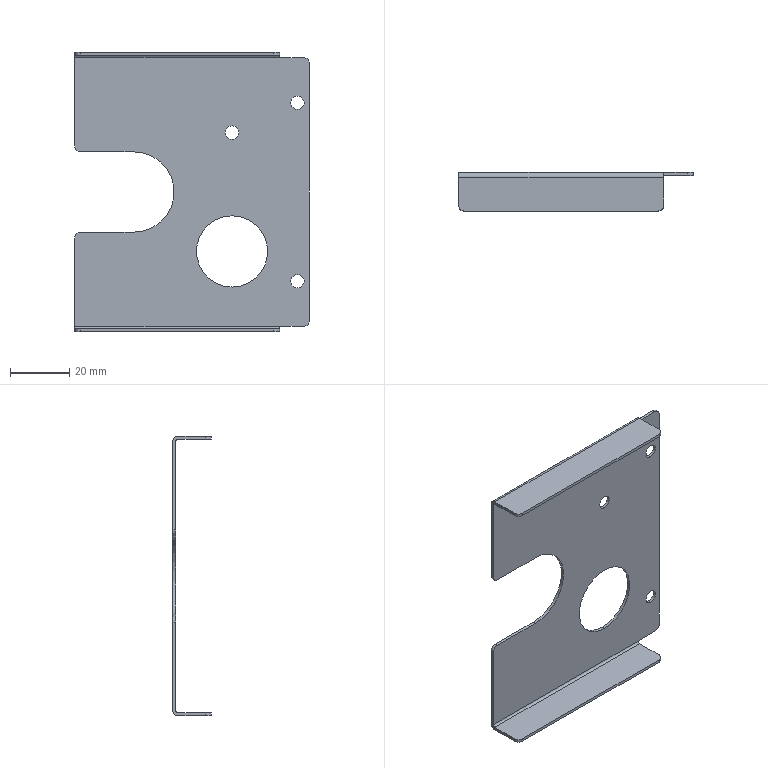Part | SolidWorks | features BaseBody 1 | 1 solid | 38 faces | box 79 x 13 x 94 mm | volume 7641 mm3 | cylinder 21 | plane 17 | commonest cylinder face diameters 4 x8 4.5 x6 1.473 x2 3.473 x2 24 x2 27 x1
STEP:
#1=CARTESIAN_POINT('',(13.5,-1.,-8.));
#2=VERTEX_POINT('',#1);
#3=CARTESIAN_POINT('',(13.5,-1.,-32.));
#4=VERTEX_POINT('',#3);
#5=CARTESIAN_POINT('',(13.5,-1.,-20.));
#6=DIRECTION('',(0.,-1.,0.));
#7=DIRECTION('',(0.,0.,1.));
#8=AXIS2_PLACEMENT_3D('',#5,#6,#7);
#9=CIRCLE('',#8,12.);
#10=EDGE_CURVE('',#2,#4,#9,.T.);
#11=ORIENTED_EDGE('',*,*,#10,.T.);
#12=CARTESIAN_POINT('',(13.5,0.,-32.));
#13=VERTEX_POINT('',#12);
#14=CARTESIAN_POINT('',(13.5,-50.,-32.));
#15=DIRECTION('',(0.,1.,0.));
#16=VECTOR('',#15,1000.);
#17=LINE('',#14,#16);
#18=EDGE_CURVE('',#4,#13,#17,.T.);
#19=ORIENTED_EDGE('',*,*,#18,.T.);
#20=CARTESIAN_POINT('',(13.5,0.,-8.));
#21=VERTEX_POINT('',#20);
#22=CARTESIAN_POINT('',(13.5,0.,-20.));
#23=DIRECTION('',(0.,-1.,0.));
#24=DIRECTION('',(0.,0.,1.));
#25=AXIS2_PLACEMENT_3D('',#22,#23,#24);
#26=CIRCLE('',#25,12.);
#27=EDGE_CURVE('',#21,#13,#26,.T.);
#28=ORIENTED_EDGE('',*,*,#27,.F.);
#29=CARTESIAN_POINT('',(13.5,-50.,-8.));
#30=DIRECTION('',(0.,1.,0.));
#31=VECTOR('',#30,1000.);
#32=LINE('',#29,#31);
#33=EDGE_CURVE('',#2,#21,#32,.T.);
#34=ORIENTED_EDGE('',*,*,#33,.F.);
#35=EDGE_LOOP('',(#11,#19,#28,#34));
#36=FACE_OUTER_BOUND('',#35,.T.);
#37=CARTESIAN_POINT('',(13.5,-50.,-20.));
#38=DIRECTION('',(0.,1.,0.));
#39=DIRECTION('',(0.,0.,1.));
#40=AXIS2_PLACEMENT_3D('',#37,#38,#39);
#41=CYLINDRICAL_SURFACE('',#40,12.);
#42=ADVANCED_FACE('',(#36),#41,.F.);
#43=CARTESIAN_POINT('',(35.5,-1.,-27.75));
#44=VERTEX_POINT('',#43);
#45=CARTESIAN_POINT('',(35.5,-1.,-32.25));
#46=VERTEX_POINT('',#45);
#47=CARTESIAN_POINT('',(35.5,-1.,-30.));
#48=DIRECTION('',(0.,-1.,0.));
#49=DIRECTION('',(0.,0.,1.));
#50=AXIS2_PLACEMENT_3D('',#47,#48,#49);
#51=CIRCLE('',#50,2.25);
#52=EDGE_CURVE('',#44,#46,#51,.T.);
#53=ORIENTED_EDGE('',*,*,#52,.T.);
#54=CARTESIAN_POINT('',(35.5,0.,-32.25));
#55=VERTEX_POINT('',#54);
#56=CARTESIAN_POINT('',(35.5,-50.,-32.25));
#57=DIRECTION('',(0.,1.,0.));
#58=VECTOR('',#57,1000.);
#59=LINE('',#56,#58);
#60=EDGE_CURVE('',#46,#55,#59,.T.);
#61=ORIENTED_EDGE('',*,*,#60,.T.);
#62=CARTESIAN_POINT('',(35.5,0.,-27.75));
#63=VERTEX_POINT('',#62);
#64=CARTESIAN_POINT('',(35.5,0.,-30.));
#65=DIRECTION('',(0.,-1.,0.));
#66=DIRECTION('',(0.,0.,1.));
#67=AXIS2_PLACEMENT_3D('',#64,#65,#66);
#68=CIRCLE('',#67,2.25);
#69=EDGE_CURVE('',#63,#55,#68,.T.);
#70=ORIENTED_EDGE('',*,*,#69,.F.);
#71=CARTESIAN_POINT('',(35.5,-50.,-27.75));
#72=DIRECTION('',(0.,1.,0.));
#73=VECTOR('',#72,1000.);
#74=LINE('',#71,#73);
#75=EDGE_CURVE('',#44,#63,#74,.T.);
#76=ORIENTED_EDGE('',*,*,#75,.F.);
#77=EDGE_LOOP('',(#53,#61,#70,#76));
#78=FACE_OUTER_BOUND('',#77,.T.);
#79=CARTESIAN_POINT('',(35.5,-50.,-30.));
#80=DIRECTION('',(0.,1.,0.));
#81=DIRECTION('',(0.,0.,1.));
#82=AXIS2_PLACEMENT_3D('',#79,#80,#81);
#83=CYLINDRICAL_SURFACE('',#82,2.25);
#84=ADVANCED_FACE('',(#78),#83,.F.);
#85=CARTESIAN_POINT('',(35.5,-1.,32.25));
#86=VERTEX_POINT('',#85);
#87=CARTESIAN_POINT('',(35.5,-1.,27.75));
#88=VERTEX_POINT('',#87);
#89=CARTESIAN_POINT('',(35.5,-1.,30.));
#90=DIRECTION('',(0.,-1.,0.));
#91=DIRECTION('',(0.,0.,1.));
#92=AXIS2_PLACEMENT_3D('',#89,#90,#91);
#93=CIRCLE('',#92,2.25);
#94=EDGE_CURVE('',#86,#88,#93,.T.);
#95=ORIENTED_EDGE('',*,*,#94,.T.);
#96=CARTESIAN_POINT('',(35.5,0.,27.75));
#97=VERTEX_POINT('',#96);
#98=CARTESIAN_POINT('',(35.5,-50.,27.75));
#99=DIRECTION('',(0.,1.,0.));
#100=VECTOR('',#99,1000.);
#101=LINE('',#98,#100);
#102=EDGE_CURVE('',#88,#97,#101,.T.);
#103=ORIENTED_EDGE('',*,*,#102,.T.);
#104=CARTESIAN_POINT('',(35.5,0.,32.25));
#105=VERTEX_POINT('',#104);
#106=CARTESIAN_POINT('',(35.5,0.,30.));
#107=DIRECTION('',(0.,-1.,0.));
#108=DIRECTION('',(0.,0.,1.));
#109=AXIS2_PLACEMENT_3D('',#106,#107,#108);
#110=CIRCLE('',#109,2.25);
#111=EDGE_CURVE('',#105,#97,#110,.T.);
#112=ORIENTED_EDGE('',*,*,#111,.F.);
#113=CARTESIAN_POINT('',(35.5,-50.,32.25));
#114=DIRECTION('',(0.,1.,0.));
#115=VECTOR('',#114,1000.);
#116=LINE('',#113,#115);
#117=EDGE_CURVE('',#86,#105,#116,.T.);
#118=ORIENTED_EDGE('',*,*,#117,.F.);
#119=EDGE_LOOP('',(#95,#103,#112,#118));
#120=FACE_OUTER_BOUND('',#119,.T.);
#121=CARTESIAN_POINT('',(35.5,-50.,30.));
#122=DIRECTION('',(0.,1.,0.));
#123=DIRECTION('',(0.,0.,1.));
#124=AXIS2_PLACEMENT_3D('',#121,#122,#123);
#125=CYLINDRICAL_SURFACE('',#124,2.25);
#126=ADVANCED_FACE('',(#120),#125,.F.);
#127=CARTESIAN_POINT('',(13.5,-1.,22.25));
#128=VERTEX_POINT('',#127);
#129=CARTESIAN_POINT('',(13.5,-1.,17.75));
#130=VERTEX_POINT('',#129);
#131=CARTESIAN_POINT('',(13.5,-1.,20.));
#132=DIRECTION('',(0.,-1.,0.));
#133=DIRECTION('',(0.,0.,1.));
#134=AXIS2_PLACEMENT_3D('',#131,#132,#133);
#135=CIRCLE('',#134,2.25);
#136=EDGE_CURVE('',#128,#130,#135,.T.);
#137=ORIENTED_EDGE('',*,*,#136,.T.);
#138=CARTESIAN_POINT('',(13.5,0.,17.75));
#139=VERTEX_POINT('',#138);
#140=CARTESIAN_POINT('',(13.5,-50.,17.75));
#141=DIRECTION('',(0.,1.,0.));
#142=VECTOR('',#141,1000.);
#143=LINE('',#140,#142);
#144=EDGE_CURVE('',#130,#139,#143,.T.);
#145=ORIENTED_EDGE('',*,*,#144,.T.);
#146=CARTESIAN_POINT('',(13.5,0.,22.25));
#147=VERTEX_POINT('',#146);
#148=CARTESIAN_POINT('',(13.5,0.,20.));
#149=DIRECTION('',(0.,-1.,0.));
#150=DIRECTION('',(0.,0.,1.));
#151=AXIS2_PLACEMENT_3D('',#148,#149,#150);
#152=CIRCLE('',#151,2.25);
#153=EDGE_CURVE('',#147,#139,#152,.T.);
#154=ORIENTED_EDGE('',*,*,#153,.F.);
#155=CARTESIAN_POINT('',(13.5,-50.,22.25));
#156=DIRECTION('',(0.,1.,0.));
#157=VECTOR('',#156,1000.);
#158=LINE('',#155,#157);
#159=EDGE_CURVE('',#128,#147,#158,.T.);
#160=ORIENTED_EDGE('',*,*,#159,.F.);
#161=EDGE_LOOP('',(#137,#145,#154,#160));
#162=FACE_OUTER_BOUND('',#161,.T.);
#163=CARTESIAN_POINT('',(13.5,-50.,20.));
#164=DIRECTION('',(0.,1.,0.));
#165=DIRECTION('',(0.,0.,1.));
#166=AXIS2_PLACEMENT_3D('',#163,#164,#165);
#167=CYLINDRICAL_SURFACE('',#166,2.25);
#168=ADVANCED_FACE('',(#162),#167,.F.);
#169=CARTESIAN_POINT('',(-39.5,-11.,-47.));
#170=VERTEX_POINT('',#169);
#171=CARTESIAN_POINT('',(-37.5,-13.,-47.));
#172=VERTEX_POINT('',#171);
#173=CARTESIAN_POINT('',(-37.5,-11.,-47.));
#174=DIRECTION('',(0.,0.,1.));
#175=DIRECTION('',(0.,-1.,0.));
#176=AXIS2_PLACEMENT_3D('',#173,#174,#175);
#177=CIRCLE('',#176,2.);
#178=EDGE_CURVE('',#170,#172,#177,.T.);
#179=ORIENTED_EDGE('',*,*,#178,.F.);
#180=CARTESIAN_POINT('',(-39.5,-1.737,-47.));
#181=VERTEX_POINT('',#180);
#182=CARTESIAN_POINT('',(-39.5,-1.,-47.));
#183=DIRECTION('',(0.,1.,0.));
#184=VECTOR('',#183,1000.);
#185=LINE('',#182,#184);
#186=EDGE_CURVE('',#170,#181,#185,.T.);
#187=ORIENTED_EDGE('',*,*,#186,.T.);
#188=CARTESIAN_POINT('',(29.5,-1.737,-47.));
#189=VERTEX_POINT('',#188);
#190=CARTESIAN_POINT('',(39.5,-1.737,-47.));
#191=DIRECTION('',(-1.,0.,0.));
#192=VECTOR('',#191,1000.);
#193=LINE('',#190,#192);
#194=EDGE_CURVE('',#189,#181,#193,.T.);
#195=ORIENTED_EDGE('',*,*,#194,.F.);
#196=CARTESIAN_POINT('',(29.5,-11.,-47.));
#197=VERTEX_POINT('',#196);
#198=CARTESIAN_POINT('',(29.5,-1.,-47.));
#199=DIRECTION('',(0.,1.,0.));
#200=VECTOR('',#199,1000.);
#201=LINE('',#198,#200);
#202=EDGE_CURVE('',#197,#189,#201,.T.);
#203=ORIENTED_EDGE('',*,*,#202,.F.);
#204=CARTESIAN_POINT('',(27.5,-13.,-47.));
#205=VERTEX_POINT('',#204);
#206=CARTESIAN_POINT('',(27.5,-11.,-47.));
#207=DIRECTION('',(0.,0.,1.));
#208=DIRECTION('',(0.,1.,0.));
#209=AXIS2_PLACEMENT_3D('',#206,#207,#208);
#210=CIRCLE('',#209,2.);
#211=EDGE_CURVE('',#205,#197,#210,.T.);
#212=ORIENTED_EDGE('',*,*,#211,.F.);
#213=CARTESIAN_POINT('',(-39.5,-13.,-47.));
#214=DIRECTION('',(-1.,0.,0.));
#215=VECTOR('',#214,1000.);
#216=LINE('',#213,#215);
#217=EDGE_CURVE('',#205,#172,#216,.T.);
#218=ORIENTED_EDGE('',*,*,#217,.T.);
#219=EDGE_LOOP('',(#179,#187,#195,#203,#212,#218));
#220=FACE_OUTER_BOUND('',#219,.T.);
#221=CARTESIAN_POINT('',(39.5,-1.,-47.));
#222=DIRECTION('',(0.,0.,1.));
#223=DIRECTION('',(0.,-1.,0.));
#224=AXIS2_PLACEMENT_3D('',#221,#222,#223);
#225=PLANE('',#224);
#226=ADVANCED_FACE('',(#220),#225,.F.);
#227=CARTESIAN_POINT('',(-37.5,-13.,47.));
#228=VERTEX_POINT('',#227);
#229=CARTESIAN_POINT('',(-39.5,-11.,47.));
#230=VERTEX_POINT('',#229);
#231=CARTESIAN_POINT('',(-37.5,-11.,47.));
#232=DIRECTION('',(0.,0.,-1.));
#233=DIRECTION('',(0.,1.,0.));
#234=AXIS2_PLACEMENT_3D('',#231,#232,#233);
#235=CIRCLE('',#234,2.);
#236=EDGE_CURVE('',#228,#230,#235,.T.);
#237=ORIENTED_EDGE('',*,*,#236,.F.);
#238=CARTESIAN_POINT('',(27.5,-13.,47.));
#239=VERTEX_POINT('',#238);
#240=CARTESIAN_POINT('',(39.5,-13.,47.));
#241=DIRECTION('',(1.,0.,0.));
#242=VECTOR('',#241,1000.);
#243=LINE('',#240,#242);
#244=EDGE_CURVE('',#228,#239,#243,.T.);
#245=ORIENTED_EDGE('',*,*,#244,.T.);
#246=CARTESIAN_POINT('',(29.5,-11.,47.));
#247=VERTEX_POINT('',#246);
#248=CARTESIAN_POINT('',(27.5,-11.,47.));
#249=DIRECTION('',(0.,0.,-1.));
#250=DIRECTION('',(0.,-1.,0.));
#251=AXIS2_PLACEMENT_3D('',#248,#249,#250);
#252=CIRCLE('',#251,2.);
#253=EDGE_CURVE('',#247,#239,#252,.T.);
#254=ORIENTED_EDGE('',*,*,#253,.F.);
#255=CARTESIAN_POINT('',(29.5,-1.737,47.));
#256=VERTEX_POINT('',#255);
#257=CARTESIAN_POINT('',(29.5,-13.,47.));
#258=DIRECTION('',(0.,-1.,0.));
#259=VECTOR('',#258,1000.);
#260=LINE('',#257,#259);
#261=EDGE_CURVE('',#256,#247,#260,.T.);
#262=ORIENTED_EDGE('',*,*,#261,.F.);
#263=CARTESIAN_POINT('',(-39.5,-1.737,47.));
#264=VERTEX_POINT('',#263);
#265=CARTESIAN_POINT('',(-39.5,-1.737,47.));
#266=DIRECTION('',(1.,0.,0.));
#267=VECTOR('',#266,1000.);
#268=LINE('',#265,#267);
#269=EDGE_CURVE('',#264,#256,#268,.T.);
#270=ORIENTED_EDGE('',*,*,#269,.F.);
#271=CARTESIAN_POINT('',(-39.5,-13.,47.));
#272=DIRECTION('',(0.,-1.,0.));
#273=VECTOR('',#272,1000.);
#274=LINE('',#271,#273);
#275=EDGE_CURVE('',#264,#230,#274,.T.);
#276=ORIENTED_EDGE('',*,*,#275,.T.);
#277=EDGE_LOOP('',(#237,#245,#254,#262,#270,#276));
#278=FACE_OUTER_BOUND('',#277,.T.);
#279=CARTESIAN_POINT('',(39.5,-13.,47.));
#280=DIRECTION('',(0.,0.,-1.));
#281=DIRECTION('',(0.,-1.,0.));
#282=AXIS2_PLACEMENT_3D('',#279,#280,#281);
#283=PLANE('',#282);
#284=ADVANCED_FACE('',(#278),#283,.F.);
#285=CARTESIAN_POINT('',(-39.5,-11.,-46.));
#286=VERTEX_POINT('',#285);
#287=CARTESIAN_POINT('',(-37.5,-13.,-46.));
#288=VERTEX_POINT('',#287);
#289=CARTESIAN_POINT('',(-37.5,-11.,-46.));
#290=DIRECTION('',(0.,0.,1.));
#291=DIRECTION('',(0.,-1.,0.));
#292=AXIS2_PLACEMENT_3D('',#289,#290,#291);
#293=CIRCLE('',#292,2.);
#294=EDGE_CURVE('',#286,#288,#293,.T.);
#295=ORIENTED_EDGE('',*,*,#294,.F.);
#296=CARTESIAN_POINT('',(-39.5,-11.,-47.));
#297=DIRECTION('',(0.,0.,-1.));
#298=VECTOR('',#297,1000.);
#299=LINE('',#296,#298);
#300=EDGE_CURVE('',#286,#170,#299,.T.);
#301=ORIENTED_EDGE('',*,*,#300,.T.);
#302=ORIENTED_EDGE('',*,*,#178,.T.);
#303=CARTESIAN_POINT('',(-37.5,-13.,-47.));
#304=DIRECTION('',(0.,0.,1.));
#305=VECTOR('',#304,1000.);
#306=LINE('',#303,#305);
#307=EDGE_CURVE('',#172,#288,#306,.T.);
#308=ORIENTED_EDGE('',*,*,#307,.T.);
#309=EDGE_LOOP('',(#295,#301,#302,#308));
#310=FACE_OUTER_BOUND('',#309,.T.);
#311=CARTESIAN_POINT('',(-37.5,-11.,-47.));
#312=DIRECTION('',(0.,0.,1.));
#313=DIRECTION('',(0.,-1.,0.));
#314=AXIS2_PLACEMENT_3D('',#311,#312,#313);
#315=CYLINDRICAL_SURFACE('',#314,2.);
#316=ADVANCED_FACE('',(#310),#315,.T.);
#317=ORIENTED_EDGE('',*,*,#307,.F.);
#318=ORIENTED_EDGE('',*,*,#217,.F.);
#319=CARTESIAN_POINT('',(27.5,-13.,-46.));
#320=VERTEX_POINT('',#319);
#321=CARTESIAN_POINT('',(27.5,-13.,-47.));
#322=DIRECTION('',(0.,0.,-1.));
#323=VECTOR('',#322,1000.);
#324=LINE('',#321,#323);
#325=EDGE_CURVE('',#320,#205,#324,.T.);
#326=ORIENTED_EDGE('',*,*,#325,.F.);
#327=CARTESIAN_POINT('',(39.5,-13.,-46.));
#328=DIRECTION('',(1.,0.,0.));
#329=VECTOR('',#328,1000.);
#330=LINE('',#327,#329);
#331=EDGE_CURVE('',#288,#320,#330,.T.);
#332=ORIENTED_EDGE('',*,*,#331,.F.);
#333=EDGE_LOOP('',(#317,#318,#326,#332));
#334=FACE_OUTER_BOUND('',#333,.T.);
#335=CARTESIAN_POINT('',(-39.5,-13.,-47.));
#336=DIRECTION('',(0.,1.,0.));
#337=DIRECTION('',(0.,0.,-1.));
#338=AXIS2_PLACEMENT_3D('',#335,#336,#337);
#339=PLANE('',#338);
#340=ADVANCED_FACE('',(#334),#339,.F.);
#341=CARTESIAN_POINT('',(29.5,-11.,-46.));
#342=VERTEX_POINT('',#341);
#343=CARTESIAN_POINT('',(27.5,-11.,-46.));
#344=DIRECTION('',(0.,0.,1.));
#345=DIRECTION('',(0.,1.,0.));
#346=AXIS2_PLACEMENT_3D('',#343,#344,#345);
#347=CIRCLE('',#346,2.);
#348=EDGE_CURVE('',#320,#342,#347,.T.);
#349=ORIENTED_EDGE('',*,*,#348,.F.);
#350=ORIENTED_EDGE('',*,*,#325,.T.);
#351=ORIENTED_EDGE('',*,*,#211,.T.);
#352=CARTESIAN_POINT('',(29.5,-11.,-47.));
#353=DIRECTION('',(0.,0.,-1.));
#354=VECTOR('',#353,1000.);
#355=LINE('',#352,#354);
#356=EDGE_CURVE('',#342,#197,#355,.T.);
#357=ORIENTED_EDGE('',*,*,#356,.F.);
#358=EDGE_LOOP('',(#349,#350,#351,#357));
#359=FACE_OUTER_BOUND('',#358,.T.);
#360=CARTESIAN_POINT('',(27.5,-11.,-47.));
#361=DIRECTION('',(0.,0.,-1.));
#362=DIRECTION('',(0.,1.,0.));
#363=AXIS2_PLACEMENT_3D('',#360,#361,#362);
#364=CYLINDRICAL_SURFACE('',#363,2.);
#365=ADVANCED_FACE('',(#359),#364,.T.);
#366=ORIENTED_EDGE('',*,*,#202,.T.);
#367=CARTESIAN_POINT('',(29.5,0.,-45.263));
#368=VERTEX_POINT('',#367);
#369=CARTESIAN_POINT('',(29.5,-1.737,-45.263));
#370=DIRECTION('',(-1.,0.,0.));
#371=DIRECTION('',(0.,0.,-1.));
#372=AXIS2_PLACEMENT_3D('',#369,#370,#371);
#373=CIRCLE('',#372,1.737);
#374=EDGE_CURVE('',#368,#189,#373,.T.);
#375=ORIENTED_EDGE('',*,*,#374,.F.);
#376=CARTESIAN_POINT('',(29.5,-1.,-45.263));
#377=VERTEX_POINT('',#376);
#378=CARTESIAN_POINT('',(29.5,-1.737,-45.263));
#379=DIRECTION('',(0.,1.,0.));
#380=VECTOR('',#379,1000.);
#381=LINE('',#378,#380);
#382=EDGE_CURVE('',#377,#368,#381,.T.);
#383=ORIENTED_EDGE('',*,*,#382,.F.);
#384=CARTESIAN_POINT('',(29.5,-1.737,-46.));
#385=VERTEX_POINT('',#384);
#386=CARTESIAN_POINT('',(29.5,-1.737,-45.263));
#387=DIRECTION('',(1.,0.,0.));
#388=DIRECTION('',(0.,0.,-1.));
#389=AXIS2_PLACEMENT_3D('',#386,#387,#388);
#390=CIRCLE('',#389,0.7366);
#391=EDGE_CURVE('',#385,#377,#390,.T.);
#392=ORIENTED_EDGE('',*,*,#391,.F.);
#393=CARTESIAN_POINT('',(29.5,-1.,-46.));
#394=DIRECTION('',(0.,1.,0.));
#395=VECTOR('',#394,1000.);
#396=LINE('',#393,#395);
#397=EDGE_CURVE('',#342,#385,#396,.T.);
#398=ORIENTED_EDGE('',*,*,#397,.F.);
#399=ORIENTED_EDGE('',*,*,#356,.T.);
#400=EDGE_LOOP('',(#366,#375,#383,#392,#398,#399));
#401=FACE_OUTER_BOUND('',#400,.T.);
#402=CARTESIAN_POINT('',(29.5,-1.,-47.));
#403=DIRECTION('',(1.,0.,0.));
#404=DIRECTION('',(0.,1.,0.));
#405=AXIS2_PLACEMENT_3D('',#402,#403,#404);
#406=PLANE('',#405);
#407=ADVANCED_FACE('',(#401),#406,.T.);
#408=CARTESIAN_POINT('',(-37.5,-13.,46.));
#409=VERTEX_POINT('',#408);
#410=CARTESIAN_POINT('',(-37.5,-13.,47.));
#411=DIRECTION('',(0.,0.,1.));
#412=VECTOR('',#411,1000.);
#413=LINE('',#410,#412);
#414=EDGE_CURVE('',#409,#228,#413,.T.);
#415=ORIENTED_EDGE('',*,*,#414,.F.);
#416=CARTESIAN_POINT('',(27.5,-13.,46.));
#417=VERTEX_POINT('',#416);
#418=CARTESIAN_POINT('',(39.5,-13.,46.));
#419=DIRECTION('',(-1.,0.,0.));
#420=VECTOR('',#419,1000.);
#421=LINE('',#418,#420);
#422=EDGE_CURVE('',#417,#409,#421,.T.);
#423=ORIENTED_EDGE('',*,*,#422,.F.);
#424=CARTESIAN_POINT('',(27.5,-13.,47.));
#425=DIRECTION('',(0.,0.,-1.));
#426=VECTOR('',#425,1000.);
#427=LINE('',#424,#426);
#428=EDGE_CURVE('',#239,#417,#427,.T.);
#429=ORIENTED_EDGE('',*,*,#428,.F.);
#430=ORIENTED_EDGE('',*,*,#244,.F.);
#431=EDGE_LOOP('',(#415,#423,#429,#430));
#432=FACE_OUTER_BOUND('',#431,.T.);
#433=CARTESIAN_POINT('',(39.5,-13.,47.));
#434=DIRECTION('',(0.,1.,0.));
#435=DIRECTION('',(0.,0.,-1.));
#436=AXIS2_PLACEMENT_3D('',#433,#434,#435);
#437=PLANE('',#436);
#438=ADVANCED_FACE('',(#432),#437,.F.);
#439=CARTESIAN_POINT('',(-39.5,-11.,46.));
#440=VERTEX_POINT('',#439);
#441=CARTESIAN_POINT('',(-37.5,-11.,46.));
#442=DIRECTION('',(0.,0.,-1.));
#443=DIRECTION('',(0.,1.,0.));
#444=AXIS2_PLACEMENT_3D('',#441,#442,#443);
#445=CIRCLE('',#444,2.);
#446=EDGE_CURVE('',#409,#440,#445,.T.);
#447=ORIENTED_EDGE('',*,*,#446,.F.);
#448=ORIENTED_EDGE('',*,*,#414,.T.);
#449=ORIENTED_EDGE('',*,*,#236,.T.);
#450=CARTESIAN_POINT('',(-39.5,-11.,47.));
#451=DIRECTION('',(0.,0.,-1.));
#452=VECTOR('',#451,1000.);
#453=LINE('',#450,#452);
#454=EDGE_CURVE('',#230,#440,#453,.T.);
#455=ORIENTED_EDGE('',*,*,#454,.T.);
#456=EDGE_LOOP('',(#447,#448,#449,#455));
#457=FACE_OUTER_BOUND('',#456,.T.);
#458=CARTESIAN_POINT('',(-37.5,-11.,47.));
#459=DIRECTION('',(0.,0.,-1.));
#460=DIRECTION('',(0.,1.,0.));
#461=AXIS2_PLACEMENT_3D('',#458,#459,#460);
#462=CYLINDRICAL_SURFACE('',#461,2.);
#463=ADVANCED_FACE('',(#457),#462,.T.);
#464=CARTESIAN_POINT('',(29.5,-1.737,46.));
#465=VERTEX_POINT('',#464);
#466=CARTESIAN_POINT('',(29.5,-11.,46.));
#467=VERTEX_POINT('',#466);
#468=CARTESIAN_POINT('',(29.5,-13.,46.));
#469=DIRECTION('',(0.,-1.,0.));
#470=VECTOR('',#469,1000.);
#471=LINE('',#468,#470);
#472=EDGE_CURVE('',#465,#467,#471,.T.);
#473=ORIENTED_EDGE('',*,*,#472,.F.);
#474=CARTESIAN_POINT('',(29.5,-1.,45.263));
#475=VERTEX_POINT('',#474);
#476=CARTESIAN_POINT('',(29.5,-1.737,45.263));
#477=DIRECTION('',(1.,0.,0.));
#478=DIRECTION('',(0.,0.,1.));
#479=AXIS2_PLACEMENT_3D('',#476,#477,#478);
#480=CIRCLE('',#479,0.7366);
#481=EDGE_CURVE('',#475,#465,#480,.T.);
#482=ORIENTED_EDGE('',*,*,#481,.F.);
#483=CARTESIAN_POINT('',(29.5,0.,45.263));
#484=VERTEX_POINT('',#483);
#485=CARTESIAN_POINT('',(29.5,-1.737,45.263));
#486=DIRECTION('',(0.,-1.,0.));
#487=VECTOR('',#486,1000.);
#488=LINE('',#485,#487);
#489=EDGE_CURVE('',#484,#475,#488,.T.);
#490=ORIENTED_EDGE('',*,*,#489,.F.);
#491=CARTESIAN_POINT('',(29.5,-1.737,45.263));
#492=DIRECTION('',(-1.,0.,0.));
#493=DIRECTION('',(0.,0.,1.));
#494=AXIS2_PLACEMENT_3D('',#491,#492,#493);
#495=CIRCLE('',#494,1.737);
#496=EDGE_CURVE('',#256,#484,#495,.T.);
#497=ORIENTED_EDGE('',*,*,#496,.F.);
#498=ORIENTED_EDGE('',*,*,#261,.T.);
#499=CARTESIAN_POINT('',(29.5,-11.,47.));
#500=DIRECTION('',(0.,0.,1.));
#501=VECTOR('',#500,1000.);
#502=LINE('',#499,#501);
#503=EDGE_CURVE('',#467,#247,#502,.T.);
#504=ORIENTED_EDGE('',*,*,#503,.F.);
#505=EDGE_LOOP('',(#473,#482,#490,#497,#498,#504));
#506=FACE_OUTER_BOUND('',#505,.T.);
#507=CARTESIAN_POINT('',(29.5,-13.,47.));
#508=DIRECTION('',(1.,0.,0.));
#509=DIRECTION('',(0.,1.,0.));
#510=AXIS2_PLACEMENT_3D('',#507,#508,#509);
#511=PLANE('',#510);
#512=ADVANCED_FACE('',(#506),#511,.T.);
#513=CARTESIAN_POINT('',(27.5,-11.,46.));
#514=DIRECTION('',(0.,0.,-1.));
#515=DIRECTION('',(0.,-1.,0.));
#516=AXIS2_PLACEMENT_3D('',#513,#514,#515);
#517=CIRCLE('',#516,2.);
#518=EDGE_CURVE('',#467,#417,#517,.T.);
#519=ORIENTED_EDGE('',*,*,#518,.F.);
#520=ORIENTED_EDGE('',*,*,#503,.T.);
#521=ORIENTED_EDGE('',*,*,#253,.T.);
#522=ORIENTED_EDGE('',*,*,#428,.T.);
#523=EDGE_LOOP('',(#519,#520,#521,#522));
#524=FACE_OUTER_BOUND('',#523,.T.);
#525=CARTESIAN_POINT('',(27.5,-11.,47.));
#526=DIRECTION('',(0.,0.,1.));
#527=DIRECTION('',(0.,-1.,0.));
#528=AXIS2_PLACEMENT_3D('',#525,#526,#527);
#529=CYLINDRICAL_SURFACE('',#528,2.);
#530=ADVANCED_FACE('',(#524),#529,.T.);
#531=ORIENTED_EDGE('',*,*,#194,.T.);
#532=CARTESIAN_POINT('',(-39.5,0.,-45.263));
#533=VERTEX_POINT('',#532);
#534=CARTESIAN_POINT('',(-39.5,-1.737,-45.263));
#535=DIRECTION('',(1.,0.,0.));
#536=DIRECTION('',(0.,0.,-1.));
#537=AXIS2_PLACEMENT_3D('',#534,#535,#536);
#538=CIRCLE('',#537,1.737);
#539=EDGE_CURVE('',#181,#533,#538,.T.);
#540=ORIENTED_EDGE('',*,*,#539,.T.);
#541=CARTESIAN_POINT('',(39.5,0.,-45.263));
#542=DIRECTION('',(-1.,0.,0.));
#543=VECTOR('',#542,1000.);
#544=LINE('',#541,#543);
#545=EDGE_CURVE('',#368,#533,#544,.T.);
#546=ORIENTED_EDGE('',*,*,#545,.F.);
#547=ORIENTED_EDGE('',*,*,#374,.T.);
#548=EDGE_LOOP('',(#531,#540,#546,#547));
#549=FACE_OUTER_BOUND('',#548,.T.);
#550=CARTESIAN_POINT('',(39.5,-1.737,-45.263));
#551=DIRECTION('',(1.,0.,0.));
#552=DIRECTION('',(0.,0.,-1.));
#553=AXIS2_PLACEMENT_3D('',#550,#551,#552);
#554=CYLINDRICAL_SURFACE('',#553,1.737);
#555=ADVANCED_FACE('',(#549),#554,.T.);
#556=CARTESIAN_POINT('',(-39.5,0.,45.263));
#557=VERTEX_POINT('',#556);
#558=CARTESIAN_POINT('',(39.5,0.,45.263));
#559=DIRECTION('',(1.,0.,0.));
#560=VECTOR('',#559,1000.);
#561=LINE('',#558,#560);
#562=EDGE_CURVE('',#557,#484,#561,.T.);
#563=ORIENTED_EDGE('',*,*,#562,.F.);
#564=CARTESIAN_POINT('',(-39.5,-1.737,45.263));
#565=DIRECTION('',(1.,0.,0.));
#566=DIRECTION('',(0.,0.,1.));
#567=AXIS2_PLACEMENT_3D('',#564,#565,#566);
#568=CIRCLE('',#567,1.737);
#569=EDGE_CURVE('',#557,#264,#568,.T.);
#570=ORIENTED_EDGE('',*,*,#569,.T.);
#571=ORIENTED_EDGE('',*,*,#269,.T.);
#572=ORIENTED_EDGE('',*,*,#496,.T.);
#573=EDGE_LOOP('',(#563,#570,#571,#572));
#574=FACE_OUTER_BOUND('',#573,.T.);
#575=CARTESIAN_POINT('',(-39.5,-1.737,45.263));
#576=DIRECTION('',(-1.,0.,0.));
#577=DIRECTION('',(0.,0.,1.));
#578=AXIS2_PLACEMENT_3D('',#575,#576,#577);
#579=CYLINDRICAL_SURFACE('',#578,1.737);
#580=ADVANCED_FACE('',(#574),#579,.T.);
#581=ORIENTED_EDGE('',*,*,#397,.T.);
#582=CARTESIAN_POINT('',(-39.5,-1.737,-46.));
#583=VERTEX_POINT('',#582);
#584=CARTESIAN_POINT('',(39.5,-1.737,-46.));
#585=DIRECTION('',(-1.,0.,0.));
#586=VECTOR('',#585,1000.);
#587=LINE('',#584,#586);
#588=EDGE_CURVE('',#385,#583,#587,.T.);
#589=ORIENTED_EDGE('',*,*,#588,.T.);
#590=CARTESIAN_POINT('',(-39.5,-1.,-46.));
#591=DIRECTION('',(0.,-1.,0.));
#592=VECTOR('',#591,1000.);
#593=LINE('',#590,#592);
#594=EDGE_CURVE('',#583,#286,#593,.T.);
#595=ORIENTED_EDGE('',*,*,#594,.T.);
#596=ORIENTED_EDGE('',*,*,#294,.T.);
#597=ORIENTED_EDGE('',*,*,#331,.T.);
#598=ORIENTED_EDGE('',*,*,#348,.T.);
#599=EDGE_LOOP('',(#581,#589,#595,#596,#597,#598));
#600=FACE_OUTER_BOUND('',#599,.T.);
#601=CARTESIAN_POINT('',(39.5,-1.,-46.));
#602=DIRECTION('',(0.,0.,1.));
#603=DIRECTION('',(0.,-1.,0.));
#604=AXIS2_PLACEMENT_3D('',#601,#602,#603);
#605=PLANE('',#604);
#606=ADVANCED_FACE('',(#600),#605,.T.);
#607=ORIENTED_EDGE('',*,*,#472,.T.);
#608=ORIENTED_EDGE('',*,*,#518,.T.);
#609=ORIENTED_EDGE('',*,*,#422,.T.);
#610=ORIENTED_EDGE('',*,*,#446,.T.);
#611=CARTESIAN_POINT('',(-39.5,-1.737,46.));
#612=VERTEX_POINT('',#611);
#613=CARTESIAN_POINT('',(-39.5,-13.,46.));
#614=DIRECTION('',(0.,1.,0.));
#615=VECTOR('',#614,1000.);
#616=LINE('',#613,#615);
#617=EDGE_CURVE('',#440,#612,#616,.T.);
#618=ORIENTED_EDGE('',*,*,#617,.T.);
#619=CARTESIAN_POINT('',(-39.5,-1.737,46.));
#620=DIRECTION('',(1.,0.,0.));
#621=VECTOR('',#620,1000.);
#622=LINE('',#619,#621);
#623=EDGE_CURVE('',#612,#465,#622,.T.);
#624=ORIENTED_EDGE('',*,*,#623,.T.);
#625=EDGE_LOOP('',(#607,#608,#609,#610,#618,#624));
#626=FACE_OUTER_BOUND('',#625,.T.);
#627=CARTESIAN_POINT('',(39.5,-13.,46.));
#628=DIRECTION('',(0.,0.,-1.));
#629=DIRECTION('',(0.,-1.,0.));
#630=AXIS2_PLACEMENT_3D('',#627,#628,#629);
#631=PLANE('',#630);
#632=ADVANCED_FACE('',(#626),#631,.T.);
#633=ORIENTED_EDGE('',*,*,#153,.T.);
#634=CARTESIAN_POINT('',(13.5,0.,20.));
#635=DIRECTION('',(0.,-1.,0.));
#636=DIRECTION('',(0.,0.,1.));
#637=AXIS2_PLACEMENT_3D('',#634,#635,#636);
#638=CIRCLE('',#637,2.25);
#639=EDGE_CURVE('',#139,#147,#638,.T.);
#640=ORIENTED_EDGE('',*,*,#639,.T.);
#641=EDGE_LOOP('',(#633,#640));
#642=FACE_BOUND('',#641,.T.);
#643=ORIENTED_EDGE('',*,*,#111,.T.);
#644=CARTESIAN_POINT('',(35.5,0.,30.));
#645=DIRECTION('',(0.,-1.,0.));
#646=DIRECTION('',(0.,0.,1.));
#647=AXIS2_PLACEMENT_3D('',#644,#645,#646);
#648=CIRCLE('',#647,2.25);
#649=EDGE_CURVE('',#97,#105,#648,.T.);
#650=ORIENTED_EDGE('',*,*,#649,.T.);
#651=EDGE_LOOP('',(#643,#650));
#652=FACE_BOUND('',#651,.T.);
#653=ORIENTED_EDGE('',*,*,#69,.T.);
#654=CARTESIAN_POINT('',(35.5,0.,-30.));
#655=DIRECTION('',(0.,-1.,0.));
#656=DIRECTION('',(0.,0.,1.));
#657=AXIS2_PLACEMENT_3D('',#654,#655,#656);
#658=CIRCLE('',#657,2.25);
#659=EDGE_CURVE('',#55,#63,#658,.T.);
#660=ORIENTED_EDGE('',*,*,#659,.T.);
#661=EDGE_LOOP('',(#653,#660));
#662=FACE_BOUND('',#661,.T.);
#663=ORIENTED_EDGE('',*,*,#27,.T.);
#664=CARTESIAN_POINT('',(13.5,0.,-20.));
#665=DIRECTION('',(0.,-1.,0.));
#666=DIRECTION('',(0.,0.,1.));
#667=AXIS2_PLACEMENT_3D('',#664,#665,#666);
#668=CIRCLE('',#667,12.);
#669=EDGE_CURVE('',#13,#21,#668,.T.);
#670=ORIENTED_EDGE('',*,*,#669,.T.);
#671=EDGE_LOOP('',(#663,#670));
#672=FACE_BOUND('',#671,.T.);
#673=CARTESIAN_POINT('',(-39.5,0.,15.5));
#674=VERTEX_POINT('',#673);
#675=CARTESIAN_POINT('',(-39.5,0.,-47.));
#676=DIRECTION('',(0.,0.,-1.));
#677=VECTOR('',#676,1000.);
#678=LINE('',#675,#677);
#679=EDGE_CURVE('',#557,#674,#678,.T.);
#680=ORIENTED_EDGE('',*,*,#679,.F.);
#681=ORIENTED_EDGE('',*,*,#562,.T.);
#682=CARTESIAN_POINT('',(37.5,0.,45.263));
#683=VERTEX_POINT('',#682);
#684=CARTESIAN_POINT('',(34.5,0.,45.263));
#685=DIRECTION('',(1.,0.,0.));
#686=VECTOR('',#685,1000.);
#687=LINE('',#684,#686);
#688=EDGE_CURVE('',#484,#683,#687,.T.);
#689=ORIENTED_EDGE('',*,*,#688,.T.);
#690=CARTESIAN_POINT('',(39.5,0.,43.263));
#691=VERTEX_POINT('',#690);
#692=CARTESIAN_POINT('',(37.5,0.,43.263));
#693=DIRECTION('',(0.,-1.,0.));
#694=DIRECTION('',(0.,0.,1.));
#695=AXIS2_PLACEMENT_3D('',#692,#693,#694);
#696=CIRCLE('',#695,2.);
#697=EDGE_CURVE('',#691,#683,#696,.T.);
#698=ORIENTED_EDGE('',*,*,#697,.F.);
#699=CARTESIAN_POINT('',(39.5,0.,-43.263));
#700=VERTEX_POINT('',#699);
#701=CARTESIAN_POINT('',(39.5,0.,-47.));
#702=DIRECTION('',(0.,0.,-1.));
#703=VECTOR('',#702,1000.);
#704=LINE('',#701,#703);
#705=EDGE_CURVE('',#691,#700,#704,.T.);
#706=ORIENTED_EDGE('',*,*,#705,.T.);
#707=CARTESIAN_POINT('',(37.5,0.,-45.263));
#708=VERTEX_POINT('',#707);
#709=CARTESIAN_POINT('',(37.5,0.,-43.263));
#710=DIRECTION('',(0.,-1.,0.));
#711=DIRECTION('',(0.,0.,1.));
#712=AXIS2_PLACEMENT_3D('',#709,#710,#711);
#713=CIRCLE('',#712,2.);
#714=EDGE_CURVE('',#708,#700,#713,.T.);
#715=ORIENTED_EDGE('',*,*,#714,.F.);
#716=CARTESIAN_POINT('',(34.5,0.,-45.263));
#717=DIRECTION('',(-1.,0.,0.));
#718=VECTOR('',#717,1000.);
#719=LINE('',#716,#718);
#720=EDGE_CURVE('',#708,#368,#719,.T.);
#721=ORIENTED_EDGE('',*,*,#720,.T.);
#722=ORIENTED_EDGE('',*,*,#545,.T.);
#723=CARTESIAN_POINT('',(-39.5,0.,-15.5));
#724=VERTEX_POINT('',#723);
#725=CARTESIAN_POINT('',(-39.5,0.,-47.));
#726=DIRECTION('',(0.,0.,-1.));
#727=VECTOR('',#726,1000.);
#728=LINE('',#725,#727);
#729=EDGE_CURVE('',#724,#533,#728,.T.);
#730=ORIENTED_EDGE('',*,*,#729,.F.);
#731=CARTESIAN_POINT('',(-37.5,0.,-13.5));
#732=VERTEX_POINT('',#731);
#733=CARTESIAN_POINT('',(-37.5,0.,-15.5));
#734=DIRECTION('',(0.,-1.,0.));
#735=DIRECTION('',(0.,0.,1.));
#736=AXIS2_PLACEMENT_3D('',#733,#734,#735);
#737=CIRCLE('',#736,2.);
#738=EDGE_CURVE('',#732,#724,#737,.T.);
#739=ORIENTED_EDGE('',*,*,#738,.F.);
#740=CARTESIAN_POINT('',(-19.5,0.,-13.5));
#741=VERTEX_POINT('',#740);
#742=CARTESIAN_POINT('',(-39.5,0.,-13.5));
#743=DIRECTION('',(1.,0.,0.));
#744=VECTOR('',#743,1000.);
#745=LINE('',#742,#744);
#746=EDGE_CURVE('',#732,#741,#745,.T.);
#747=ORIENTED_EDGE('',*,*,#746,.T.);
#748=CARTESIAN_POINT('',(-19.5,0.,13.5));
#749=VERTEX_POINT('',#748);
#750=CARTESIAN_POINT('',(-19.5,0.,0.));
#751=DIRECTION('',(0.,-1.,0.));
#752=DIRECTION('',(0.,0.,1.));
#753=AXIS2_PLACEMENT_3D('',#750,#751,#752);
#754=CIRCLE('',#753,13.5);
#755=EDGE_CURVE('',#741,#749,#754,.T.);
#756=ORIENTED_EDGE('',*,*,#755,.T.);
#757=CARTESIAN_POINT('',(-37.5,0.,13.5));
#758=VERTEX_POINT('',#757);
#759=CARTESIAN_POINT('',(-19.5,0.,13.5));
#760=DIRECTION('',(-1.,0.,0.));
#761=VECTOR('',#760,1000.);
#762=LINE('',#759,#761);
#763=EDGE_CURVE('',#749,#758,#762,.T.);
#764=ORIENTED_EDGE('',*,*,#763,.T.);
#765=CARTESIAN_POINT('',(-37.5,0.,15.5));
#766=DIRECTION('',(0.,-1.,0.));
#767=DIRECTION('',(0.,0.,-1.));
#768=AXIS2_PLACEMENT_3D('',#765,#766,#767);
#769=CIRCLE('',#768,2.);
#770=EDGE_CURVE('',#674,#758,#769,.T.);
#771=ORIENTED_EDGE('',*,*,#770,.F.);
#772=EDGE_LOOP('',(#680,#681,#689,#698,#706,#715,#721,#722,#730,#739,#747,#756,#764,#771));
#773=FACE_OUTER_BOUND('',#772,.T.);
#774=CARTESIAN_POINT('',(39.5,0.,47.));
#775=DIRECTION('',(0.,1.,0.));
#776=DIRECTION('',(1.,0.,0.));
#777=AXIS2_PLACEMENT_3D('',#774,#775,#776);
#778=PLANE('',#777);
#779=ADVANCED_FACE('',(#642,#652,#662,#672,#773),#778,.T.);
#780=ORIENTED_EDGE('',*,*,#714,.T.);
#781=CARTESIAN_POINT('',(39.5,-1.,-43.263));
#782=VERTEX_POINT('',#781);
#783=CARTESIAN_POINT('',(39.5,-1.,-43.263));
#784=DIRECTION('',(0.,-1.,0.));
#785=VECTOR('',#784,1000.);
#786=LINE('',#783,#785);
#787=EDGE_CURVE('',#700,#782,#786,.T.);
#788=ORIENTED_EDGE('',*,*,#787,.T.);
#789=CARTESIAN_POINT('',(37.5,-1.,-45.263));
#790=VERTEX_POINT('',#789);
#791=CARTESIAN_POINT('',(37.5,-1.,-43.263));
#792=DIRECTION('',(0.,1.,0.));
#793=DIRECTION('',(0.,0.,1.));
#794=AXIS2_PLACEMENT_3D('',#791,#792,#793);
#795=CIRCLE('',#794,2.);
#796=EDGE_CURVE('',#782,#790,#795,.T.);
#797=ORIENTED_EDGE('',*,*,#796,.T.);
#798=CARTESIAN_POINT('',(37.5,-1.,-45.263));
#799=DIRECTION('',(0.,1.,0.));
#800=VECTOR('',#799,1000.);
#801=LINE('',#798,#800);
#802=EDGE_CURVE('',#790,#708,#801,.T.);
#803=ORIENTED_EDGE('',*,*,#802,.T.);
#804=EDGE_LOOP('',(#780,#788,#797,#803));
#805=FACE_OUTER_BOUND('',#804,.T.);
#806=CARTESIAN_POINT('',(37.5,-1.,-43.263));
#807=DIRECTION('',(0.,1.,0.));
#808=DIRECTION('',(0.,0.,1.));
#809=AXIS2_PLACEMENT_3D('',#806,#807,#808);
#810=CYLINDRICAL_SURFACE('',#809,2.);
#811=ADVANCED_FACE('',(#805),#810,.T.);
#812=ORIENTED_EDGE('',*,*,#802,.F.);
#813=CARTESIAN_POINT('',(39.5,-1.,-45.263));
#814=DIRECTION('',(-1.,0.,0.));
#815=VECTOR('',#814,1000.);
#816=LINE('',#813,#815);
#817=EDGE_CURVE('',#790,#377,#816,.T.);
#818=ORIENTED_EDGE('',*,*,#817,.T.);
#819=ORIENTED_EDGE('',*,*,#382,.T.);
#820=ORIENTED_EDGE('',*,*,#720,.F.);
#821=EDGE_LOOP('',(#812,#818,#819,#820));
#822=FACE_OUTER_BOUND('',#821,.T.);
#823=CARTESIAN_POINT('',(34.5,-1.,-45.263));
#824=DIRECTION('',(0.,0.,1.));
#825=DIRECTION('',(1.,0.,0.));
#826=AXIS2_PLACEMENT_3D('',#823,#824,#825);
#827=PLANE('',#826);
#828=ADVANCED_FACE('',(#822),#827,.F.);
#829=CARTESIAN_POINT('',(-39.5,-1.,-45.263));
#830=VERTEX_POINT('',#829);
#831=CARTESIAN_POINT('',(39.5,-1.,-45.263));
#832=DIRECTION('',(-1.,0.,0.));
#833=VECTOR('',#832,1000.);
#834=LINE('',#831,#833);
#835=EDGE_CURVE('',#377,#830,#834,.T.);
#836=ORIENTED_EDGE('',*,*,#835,.T.);
#837=CARTESIAN_POINT('',(-39.5,-1.737,-45.263));
#838=DIRECTION('',(1.,0.,0.));
#839=DIRECTION('',(0.,0.,-1.));
#840=AXIS2_PLACEMENT_3D('',#837,#838,#839);
#841=CIRCLE('',#840,0.7366);
#842=EDGE_CURVE('',#583,#830,#841,.T.);
#843=ORIENTED_EDGE('',*,*,#842,.F.);
#844=ORIENTED_EDGE('',*,*,#588,.F.);
#845=ORIENTED_EDGE('',*,*,#391,.T.);
#846=EDGE_LOOP('',(#836,#843,#844,#845));
#847=FACE_OUTER_BOUND('',#846,.T.);
#848=CARTESIAN_POINT('',(39.5,-1.737,-45.263));
#849=DIRECTION('',(1.,0.,0.));
#850=DIRECTION('',(0.,0.,-1.));
#851=AXIS2_PLACEMENT_3D('',#848,#849,#850);
#852=CYLINDRICAL_SURFACE('',#851,0.7366);
#853=ADVANCED_FACE('',(#847),#852,.F.);
#854=ORIENTED_EDGE('',*,*,#729,.T.);
#855=ORIENTED_EDGE('',*,*,#539,.F.);
#856=ORIENTED_EDGE('',*,*,#186,.F.);
#857=ORIENTED_EDGE('',*,*,#300,.F.);
#858=ORIENTED_EDGE('',*,*,#594,.F.);
#859=ORIENTED_EDGE('',*,*,#842,.T.);
#860=CARTESIAN_POINT('',(-39.5,-1.,-15.5));
#861=VERTEX_POINT('',#860);
#862=CARTESIAN_POINT('',(-39.5,-1.,47.));
#863=DIRECTION('',(0.,0.,1.));
#864=VECTOR('',#863,1000.);
#865=LINE('',#862,#864);
#866=EDGE_CURVE('',#830,#861,#865,.T.);
#867=ORIENTED_EDGE('',*,*,#866,.T.);
#868=CARTESIAN_POINT('',(-39.5,-50.,-15.5));
#869=DIRECTION('',(0.,-1.,0.));
#870=VECTOR('',#869,1000.);
#871=LINE('',#868,#870);
#872=EDGE_CURVE('',#724,#861,#871,.T.);
#873=ORIENTED_EDGE('',*,*,#872,.F.);
#874=EDGE_LOOP('',(#854,#855,#856,#857,#858,#859,#867,#873));
#875=FACE_OUTER_BOUND('',#874,.T.);
#876=CARTESIAN_POINT('',(-39.5,-1.,-47.));
#877=DIRECTION('',(-1.,0.,0.));
#878=DIRECTION('',(0.,0.,1.));
#879=AXIS2_PLACEMENT_3D('',#876,#877,#878);
#880=PLANE('',#879);
#881=ADVANCED_FACE('',(#875),#880,.T.);
#882=CARTESIAN_POINT('',(-37.5,-1.,-13.5));
#883=VERTEX_POINT('',#882);
#884=CARTESIAN_POINT('',(-37.5,-1.,-15.5));
#885=DIRECTION('',(0.,1.,0.));
#886=DIRECTION('',(0.,0.,1.));
#887=AXIS2_PLACEMENT_3D('',#884,#885,#886);
#888=CIRCLE('',#887,2.);
#889=EDGE_CURVE('',#861,#883,#888,.T.);
#890=ORIENTED_EDGE('',*,*,#889,.T.);
#891=CARTESIAN_POINT('',(-37.5,-50.,-13.5));
#892=DIRECTION('',(0.,1.,0.));
#893=VECTOR('',#892,1000.);
#894=LINE('',#891,#893);
#895=EDGE_CURVE('',#883,#732,#894,.T.);
#896=ORIENTED_EDGE('',*,*,#895,.T.);
#897=ORIENTED_EDGE('',*,*,#738,.T.);
#898=ORIENTED_EDGE('',*,*,#872,.T.);
#899=EDGE_LOOP('',(#890,#896,#897,#898));
#900=FACE_OUTER_BOUND('',#899,.T.);
#901=CARTESIAN_POINT('',(-37.5,-50.,-15.5));
#902=DIRECTION('',(0.,1.,0.));
#903=DIRECTION('',(0.,0.,1.));
#904=AXIS2_PLACEMENT_3D('',#901,#902,#903);
#905=CYLINDRICAL_SURFACE('',#904,2.);
#906=ADVANCED_FACE('',(#900),#905,.T.);
#907=ORIENTED_EDGE('',*,*,#895,.F.);
#908=CARTESIAN_POINT('',(-19.5,-1.,-13.5));
#909=VERTEX_POINT('',#908);
#910=CARTESIAN_POINT('',(39.5,-1.,-13.5));
#911=DIRECTION('',(1.,0.,0.));
#912=VECTOR('',#911,1000.);
#913=LINE('',#910,#912);
#914=EDGE_CURVE('',#883,#909,#913,.T.);
#915=ORIENTED_EDGE('',*,*,#914,.T.);
#916=CARTESIAN_POINT('',(-19.5,-50.,-13.5));
#917=DIRECTION('',(0.,1.,0.));
#918=VECTOR('',#917,1000.);
#919=LINE('',#916,#918);
#920=EDGE_CURVE('',#909,#741,#919,.T.);
#921=ORIENTED_EDGE('',*,*,#920,.T.);
#922=ORIENTED_EDGE('',*,*,#746,.F.);
#923=EDGE_LOOP('',(#907,#915,#921,#922));
#924=FACE_OUTER_BOUND('',#923,.T.);
#925=CARTESIAN_POINT('',(-39.5,-50.,-13.5));
#926=DIRECTION('',(0.,0.,-1.));
#927=DIRECTION('',(0.,-1.,0.));
#928=AXIS2_PLACEMENT_3D('',#925,#926,#927);
#929=PLANE('',#928);
#930=ADVANCED_FACE('',(#924),#929,.F.);
#931=ORIENTED_EDGE('',*,*,#755,.F.);
#932=ORIENTED_EDGE('',*,*,#920,.F.);
#933=CARTESIAN_POINT('',(-19.5,-1.,13.5));
#934=VERTEX_POINT('',#933);
#935=CARTESIAN_POINT('',(-19.5,-1.,0.));
#936=DIRECTION('',(0.,-1.,0.));
#937=DIRECTION('',(0.,0.,1.));
#938=AXIS2_PLACEMENT_3D('',#935,#936,#937);
#939=CIRCLE('',#938,13.5);
#940=EDGE_CURVE('',#909,#934,#939,.T.);
#941=ORIENTED_EDGE('',*,*,#940,.T.);
#942=CARTESIAN_POINT('',(-19.5,-50.,13.5));
#943=DIRECTION('',(0.,1.,0.));
#944=VECTOR('',#943,1000.);
#945=LINE('',#942,#944);
#946=EDGE_CURVE('',#934,#749,#945,.T.);
#947=ORIENTED_EDGE('',*,*,#946,.T.);
#948=EDGE_LOOP('',(#931,#932,#941,#947));
#949=FACE_OUTER_BOUND('',#948,.T.);
#950=CARTESIAN_POINT('',(-19.5,-50.,0.));
#951=DIRECTION('',(0.,1.,0.));
#952=DIRECTION('',(0.,0.,1.));
#953=AXIS2_PLACEMENT_3D('',#950,#951,#952);
#954=CYLINDRICAL_SURFACE('',#953,13.5);
#955=ADVANCED_FACE('',(#949),#954,.F.);
#956=CARTESIAN_POINT('',(-37.5,-1.,13.5));
#957=VERTEX_POINT('',#956);
#958=CARTESIAN_POINT('',(-37.5,-50.,13.5));
#959=DIRECTION('',(0.,-1.,0.));
#960=VECTOR('',#959,1000.);
#961=LINE('',#958,#960);
#962=EDGE_CURVE('',#758,#957,#961,.T.);
#963=ORIENTED_EDGE('',*,*,#962,.F.);
#964=ORIENTED_EDGE('',*,*,#763,.F.);
#965=ORIENTED_EDGE('',*,*,#946,.F.);
#966=CARTESIAN_POINT('',(39.5,-1.,13.5));
#967=DIRECTION('',(-1.,0.,0.));
#968=VECTOR('',#967,1000.);
#969=LINE('',#966,#968);
#970=EDGE_CURVE('',#934,#957,#969,.T.);
#971=ORIENTED_EDGE('',*,*,#970,.T.);
#972=EDGE_LOOP('',(#963,#964,#965,#971));
#973=FACE_OUTER_BOUND('',#972,.T.);
#974=CARTESIAN_POINT('',(-19.5,-50.,13.5));
#975=DIRECTION('',(0.,0.,1.));
#976=DIRECTION('',(1.,0.,0.));
#977=AXIS2_PLACEMENT_3D('',#974,#975,#976);
#978=PLANE('',#977);
#979=ADVANCED_FACE('',(#973),#978,.F.);
#980=ORIENTED_EDGE('',*,*,#770,.T.);
#981=ORIENTED_EDGE('',*,*,#962,.T.);
#982=CARTESIAN_POINT('',(-39.5,-1.,15.5));
#983=VERTEX_POINT('',#982);
#984=CARTESIAN_POINT('',(-37.5,-1.,15.5));
#985=DIRECTION('',(0.,1.,0.));
#986=DIRECTION('',(0.,0.,-1.));
#987=AXIS2_PLACEMENT_3D('',#984,#985,#986);
#988=CIRCLE('',#987,2.);
#989=EDGE_CURVE('',#957,#983,#988,.T.);
#990=ORIENTED_EDGE('',*,*,#989,.T.);
#991=CARTESIAN_POINT('',(-39.5,-1.,15.5));
#992=DIRECTION('',(0.,-1.,0.));
#993=VECTOR('',#992,1000.);
#994=LINE('',#991,#993);
#995=EDGE_CURVE('',#674,#983,#994,.T.);
#996=ORIENTED_EDGE('',*,*,#995,.F.);
#997=EDGE_LOOP('',(#980,#981,#990,#996));
#998=FACE_OUTER_BOUND('',#997,.T.);
#999=CARTESIAN_POINT('',(-37.5,-50.,15.5));
#1000=DIRECTION('',(0.,-1.,0.));
#1001=DIRECTION('',(0.,0.,-1.));
#1002=AXIS2_PLACEMENT_3D('',#999,#1000,#1001);
#1003=CYLINDRICAL_SURFACE('',#1002,2.);
#1004=ADVANCED_FACE('',(#998),#1003,.T.);
#1005=CARTESIAN_POINT('',(-39.5,-1.,45.263));
#1006=VERTEX_POINT('',#1005);
#1007=CARTESIAN_POINT('',(-39.5,-1.,47.));
#1008=DIRECTION('',(0.,0.,1.));
#1009=VECTOR('',#1008,1000.);
#1010=LINE('',#1007,#1009);
#1011=EDGE_CURVE('',#983,#1006,#1010,.T.);
#1012=ORIENTED_EDGE('',*,*,#1011,.T.);
#1013=CARTESIAN_POINT('',(-39.5,-1.737,45.263));
#1014=DIRECTION('',(-1.,0.,0.));
#1015=DIRECTION('',(0.,0.,1.));
#1016=AXIS2_PLACEMENT_3D('',#1013,#1014,#1015);
#1017=CIRCLE('',#1016,0.7366);
#1018=EDGE_CURVE('',#612,#1006,#1017,.T.);
#1019=ORIENTED_EDGE('',*,*,#1018,.F.);
#1020=ORIENTED_EDGE('',*,*,#617,.F.);
#1021=ORIENTED_EDGE('',*,*,#454,.F.);
#1022=ORIENTED_EDGE('',*,*,#275,.F.);
#1023=ORIENTED_EDGE('',*,*,#569,.F.);
#1024=ORIENTED_EDGE('',*,*,#679,.T.);
#1025=ORIENTED_EDGE('',*,*,#995,.T.);
#1026=EDGE_LOOP('',(#1012,#1019,#1020,#1021,#1022,#1023,#1024,#1025));
#1027=FACE_OUTER_BOUND('',#1026,.T.);
#1028=CARTESIAN_POINT('',(-39.5,-1.,-47.));
#1029=DIRECTION('',(-1.,0.,0.));
#1030=DIRECTION('',(0.,0.,1.));
#1031=AXIS2_PLACEMENT_3D('',#1028,#1029,#1030);
#1032=PLANE('',#1031);
#1033=ADVANCED_FACE('',(#1027),#1032,.T.);
#1034=ORIENTED_EDGE('',*,*,#623,.F.);
#1035=ORIENTED_EDGE('',*,*,#1018,.T.);
#1036=CARTESIAN_POINT('',(39.5,-1.,45.263));
#1037=DIRECTION('',(1.,0.,0.));
#1038=VECTOR('',#1037,1000.);
#1039=LINE('',#1036,#1038);
#1040=EDGE_CURVE('',#1006,#475,#1039,.T.);
#1041=ORIENTED_EDGE('',*,*,#1040,.T.);
#1042=ORIENTED_EDGE('',*,*,#481,.T.);
#1043=EDGE_LOOP('',(#1034,#1035,#1041,#1042));
#1044=FACE_OUTER_BOUND('',#1043,.T.);
#1045=CARTESIAN_POINT('',(-39.5,-1.737,45.263));
#1046=DIRECTION('',(-1.,0.,0.));
#1047=DIRECTION('',(0.,0.,1.));
#1048=AXIS2_PLACEMENT_3D('',#1045,#1046,#1047);
#1049=CYLINDRICAL_SURFACE('',#1048,0.7366);
#1050=ADVANCED_FACE('',(#1044),#1049,.F.);
#1051=CARTESIAN_POINT('',(37.5,-1.,45.263));
#1052=VERTEX_POINT('',#1051);
#1053=CARTESIAN_POINT('',(37.5,-1.,45.263));
#1054=DIRECTION('',(0.,-1.,0.));
#1055=VECTOR('',#1054,1000.);
#1056=LINE('',#1053,#1055);
#1057=EDGE_CURVE('',#683,#1052,#1056,.T.);
#1058=ORIENTED_EDGE('',*,*,#1057,.F.);
#1059=ORIENTED_EDGE('',*,*,#688,.F.);
#1060=ORIENTED_EDGE('',*,*,#489,.T.);
#1061=CARTESIAN_POINT('',(39.5,-1.,45.263));
#1062=DIRECTION('',(1.,0.,0.));
#1063=VECTOR('',#1062,1000.);
#1064=LINE('',#1061,#1063);
#1065=EDGE_CURVE('',#475,#1052,#1064,.T.);
#1066=ORIENTED_EDGE('',*,*,#1065,.T.);
#1067=EDGE_LOOP('',(#1058,#1059,#1060,#1066));
#1068=FACE_OUTER_BOUND('',#1067,.T.);
#1069=CARTESIAN_POINT('',(34.5,-1.,45.263));
#1070=DIRECTION('',(0.,0.,-1.));
#1071=DIRECTION('',(0.,-1.,0.));
#1072=AXIS2_PLACEMENT_3D('',#1069,#1070,#1071);
#1073=PLANE('',#1072);
#1074=ADVANCED_FACE('',(#1068),#1073,.F.);
#1075=ORIENTED_EDGE('',*,*,#697,.T.);
#1076=ORIENTED_EDGE('',*,*,#1057,.T.);
#1077=CARTESIAN_POINT('',(39.5,-1.,43.263));
#1078=VERTEX_POINT('',#1077);
#1079=CARTESIAN_POINT('',(37.5,-1.,43.263));
#1080=DIRECTION('',(0.,1.,0.));
#1081=DIRECTION('',(0.,0.,1.));
#1082=AXIS2_PLACEMENT_3D('',#1079,#1080,#1081);
#1083=CIRCLE('',#1082,2.);
#1084=EDGE_CURVE('',#1052,#1078,#1083,.T.);
#1085=ORIENTED_EDGE('',*,*,#1084,.T.);
#1086=CARTESIAN_POINT('',(39.5,-1.,43.263));
#1087=DIRECTION('',(0.,1.,0.));
#1088=VECTOR('',#1087,1000.);
#1089=LINE('',#1086,#1088);
#1090=EDGE_CURVE('',#1078,#691,#1089,.T.);
#1091=ORIENTED_EDGE('',*,*,#1090,.T.);
#1092=EDGE_LOOP('',(#1075,#1076,#1085,#1091));
#1093=FACE_OUTER_BOUND('',#1092,.T.);
#1094=CARTESIAN_POINT('',(37.5,-1.,43.263));
#1095=DIRECTION('',(0.,1.,0.));
#1096=DIRECTION('',(0.,0.,1.));
#1097=AXIS2_PLACEMENT_3D('',#1094,#1095,#1096);
#1098=CYLINDRICAL_SURFACE('',#1097,2.);
#1099=ADVANCED_FACE('',(#1093),#1098,.T.);
#1100=ORIENTED_EDGE('',*,*,#1090,.F.);
#1101=CARTESIAN_POINT('',(39.5,-1.,47.));
#1102=DIRECTION('',(0.,0.,-1.));
#1103=VECTOR('',#1102,1000.);
#1104=LINE('',#1101,#1103);
#1105=EDGE_CURVE('',#1078,#782,#1104,.T.);
#1106=ORIENTED_EDGE('',*,*,#1105,.T.);
#1107=ORIENTED_EDGE('',*,*,#787,.F.);
#1108=ORIENTED_EDGE('',*,*,#705,.F.);
#1109=EDGE_LOOP('',(#1100,#1106,#1107,#1108));
#1110=FACE_OUTER_BOUND('',#1109,.T.);
#1111=CARTESIAN_POINT('',(39.5,-1.,-47.));
#1112=DIRECTION('',(-1.,0.,0.));
#1113=DIRECTION('',(0.,0.,1.));
#1114=AXIS2_PLACEMENT_3D('',#1111,#1112,#1113);
#1115=PLANE('',#1114);
#1116=ADVANCED_FACE('',(#1110),#1115,.F.);
#1117=ORIENTED_EDGE('',*,*,#136,.F.);
#1118=CARTESIAN_POINT('',(13.5,-1.,20.));
#1119=DIRECTION('',(0.,-1.,0.));
#1120=DIRECTION('',(0.,0.,1.));
#1121=AXIS2_PLACEMENT_3D('',#1118,#1119,#1120);
#1122=CIRCLE('',#1121,2.25);
#1123=EDGE_CURVE('',#130,#128,#1122,.T.);
#1124=ORIENTED_EDGE('',*,*,#1123,.F.);
#1125=EDGE_LOOP('',(#1117,#1124));
#1126=FACE_BOUND('',#1125,.T.);
#1127=ORIENTED_EDGE('',*,*,#94,.F.);
#1128=CARTESIAN_POINT('',(35.5,-1.,30.));
#1129=DIRECTION('',(0.,-1.,0.));
#1130=DIRECTION('',(0.,0.,1.));
#1131=AXIS2_PLACEMENT_3D('',#1128,#1129,#1130);
#1132=CIRCLE('',#1131,2.25);
#1133=EDGE_CURVE('',#88,#86,#1132,.T.);
#1134=ORIENTED_EDGE('',*,*,#1133,.F.);
#1135=EDGE_LOOP('',(#1127,#1134));
#1136=FACE_BOUND('',#1135,.T.);
#1137=ORIENTED_EDGE('',*,*,#52,.F.);
#1138=CARTESIAN_POINT('',(35.5,-1.,-30.));
#1139=DIRECTION('',(0.,-1.,0.));
#1140=DIRECTION('',(0.,0.,1.));
#1141=AXIS2_PLACEMENT_3D('',#1138,#1139,#1140);
#1142=CIRCLE('',#1141,2.25);
#1143=EDGE_CURVE('',#46,#44,#1142,.T.);
#1144=ORIENTED_EDGE('',*,*,#1143,.F.);
#1145=EDGE_LOOP('',(#1137,#1144));
#1146=FACE_BOUND('',#1145,.T.);
#1147=ORIENTED_EDGE('',*,*,#10,.F.);
#1148=CARTESIAN_POINT('',(13.5,-1.,-20.));
#1149=DIRECTION('',(0.,-1.,0.));
#1150=DIRECTION('',(0.,0.,1.));
#1151=AXIS2_PLACEMENT_3D('',#1148,#1149,#1150);
#1152=CIRCLE('',#1151,12.);
#1153=EDGE_CURVE('',#4,#2,#1152,.T.);
#1154=ORIENTED_EDGE('',*,*,#1153,.F.);
#1155=EDGE_LOOP('',(#1147,#1154));
#1156=FACE_BOUND('',#1155,.T.);
#1157=ORIENTED_EDGE('',*,*,#1084,.F.);
#1158=ORIENTED_EDGE('',*,*,#1065,.F.);
#1159=ORIENTED_EDGE('',*,*,#1040,.F.);
#1160=ORIENTED_EDGE('',*,*,#1011,.F.);
#1161=ORIENTED_EDGE('',*,*,#989,.F.);
#1162=ORIENTED_EDGE('',*,*,#970,.F.);
#1163=ORIENTED_EDGE('',*,*,#940,.F.);
#1164=ORIENTED_EDGE('',*,*,#914,.F.);
#1165=ORIENTED_EDGE('',*,*,#889,.F.);
#1166=ORIENTED_EDGE('',*,*,#866,.F.);
#1167=ORIENTED_EDGE('',*,*,#835,.F.);
#1168=ORIENTED_EDGE('',*,*,#817,.F.);
#1169=ORIENTED_EDGE('',*,*,#796,.F.);
#1170=ORIENTED_EDGE('',*,*,#1105,.F.);
#1171=EDGE_LOOP('',(#1157,#1158,#1159,#1160,#1161,#1162,#1163,#1164,#1165,#1166,#1167,#1168,#1169,#1170));
#1172=FACE_OUTER_BOUND('',#1171,.T.);
#1173=CARTESIAN_POINT('',(39.5,-1.,47.));
#1174=DIRECTION('',(0.,1.,0.));
#1175=DIRECTION('',(1.,0.,0.));
#1176=AXIS2_PLACEMENT_3D('',#1173,#1174,#1175);
#1177=PLANE('',#1176);
#1178=ADVANCED_FACE('',(#1126,#1136,#1146,#1156,#1172),#1177,.F.);
#1179=ORIENTED_EDGE('',*,*,#144,.F.);
#1180=ORIENTED_EDGE('',*,*,#1123,.T.);
#1181=ORIENTED_EDGE('',*,*,#159,.T.);
#1182=ORIENTED_EDGE('',*,*,#639,.F.);
#1183=EDGE_LOOP('',(#1179,#1180,#1181,#1182));
#1184=FACE_OUTER_BOUND('',#1183,.T.);
#1185=CARTESIAN_POINT('',(13.5,-50.,20.));
#1186=DIRECTION('',(0.,1.,0.));
#1187=DIRECTION('',(0.,0.,1.));
#1188=AXIS2_PLACEMENT_3D('',#1185,#1186,#1187);
#1189=CYLINDRICAL_SURFACE('',#1188,2.25);
#1190=ADVANCED_FACE('',(#1184),#1189,.F.);
#1191=ORIENTED_EDGE('',*,*,#102,.F.);
#1192=ORIENTED_EDGE('',*,*,#1133,.T.);
#1193=ORIENTED_EDGE('',*,*,#117,.T.);
#1194=ORIENTED_EDGE('',*,*,#649,.F.);
#1195=EDGE_LOOP('',(#1191,#1192,#1193,#1194));
#1196=FACE_OUTER_BOUND('',#1195,.T.);
#1197=CARTESIAN_POINT('',(35.5,-50.,30.));
#1198=DIRECTION('',(0.,1.,0.));
#1199=DIRECTION('',(0.,0.,1.));
#1200=AXIS2_PLACEMENT_3D('',#1197,#1198,#1199);
#1201=CYLINDRICAL_SURFACE('',#1200,2.25);
#1202=ADVANCED_FACE('',(#1196),#1201,.F.);
#1203=ORIENTED_EDGE('',*,*,#60,.F.);
#1204=ORIENTED_EDGE('',*,*,#1143,.T.);
#1205=ORIENTED_EDGE('',*,*,#75,.T.);
#1206=ORIENTED_EDGE('',*,*,#659,.F.);
#1207=EDGE_LOOP('',(#1203,#1204,#1205,#1206));
#1208=FACE_OUTER_BOUND('',#1207,.T.);
#1209=CARTESIAN_POINT('',(35.5,-50.,-30.));
#1210=DIRECTION('',(0.,1.,0.));
#1211=DIRECTION('',(0.,0.,1.));
#1212=AXIS2_PLACEMENT_3D('',#1209,#1210,#1211);
#1213=CYLINDRICAL_SURFACE('',#1212,2.25);
#1214=ADVANCED_FACE('',(#1208),#1213,.F.);
#1215=ORIENTED_EDGE('',*,*,#18,.F.);
#1216=ORIENTED_EDGE('',*,*,#1153,.T.);
#1217=ORIENTED_EDGE('',*,*,#33,.T.);
#1218=ORIENTED_EDGE('',*,*,#669,.F.);
#1219=EDGE_LOOP('',(#1215,#1216,#1217,#1218));
#1220=FACE_OUTER_BOUND('',#1219,.T.);
#1221=CARTESIAN_POINT('',(13.5,-50.,-20.));
#1222=DIRECTION('',(0.,1.,0.));
#1223=DIRECTION('',(0.,0.,1.));
#1224=AXIS2_PLACEMENT_3D('',#1221,#1222,#1223);
#1225=CYLINDRICAL_SURFACE('',#1224,12.);
#1226=ADVANCED_FACE('',(#1220),#1225,.F.);
#1227=CLOSED_SHELL('',(#42,#84,#126,#168,#226,#284,#316,#340,#365,#407,#438,#463,#512,#530,#555,#580,#606,#632,#779,#811,#828,#853,#881,#906,#930,#955,#979,#1004,#1033,#1050,#1074,#1099,#1116,#1178,#1190,#1202,#1214,#1226));
#1228=MANIFOLD_SOLID_BREP('',#1227);
#1229=CARTESIAN_POINT('',(0.,0.,0.));
#1230=DIRECTION('',(0.,0.,1.));
#1231=DIRECTION('',(1.,0.,0.));
#1232=AXIS2_PLACEMENT_3D('',#1229,#1230,#1231);
#1233=(LENGTH_UNIT()NAMED_UNIT(*)SI_UNIT(.MILLI.,.METRE.));
#1234=UNCERTAINTY_MEASURE_WITH_UNIT(LENGTH_MEASURE(0.00001),#1233,'','');
#1235=(NAMED_UNIT(*)PLANE_ANGLE_UNIT()SI_UNIT($,.RADIAN.));
#1236=(NAMED_UNIT(*)SI_UNIT($,.STERADIAN.)SOLID_ANGLE_UNIT());
#1237=(GEOMETRIC_REPRESENTATION_CONTEXT(3)GLOBAL_UNCERTAINTY_ASSIGNED_CONTEXT((#1234))GLOBAL_UNIT_ASSIGNED_CONTEXT((#1233,#1235,#1236))REPRESENTATION_CONTEXT('',''));
#1238=ADVANCED_BREP_SHAPE_REPRESENTATION('',(#1228,#1232),#1237);